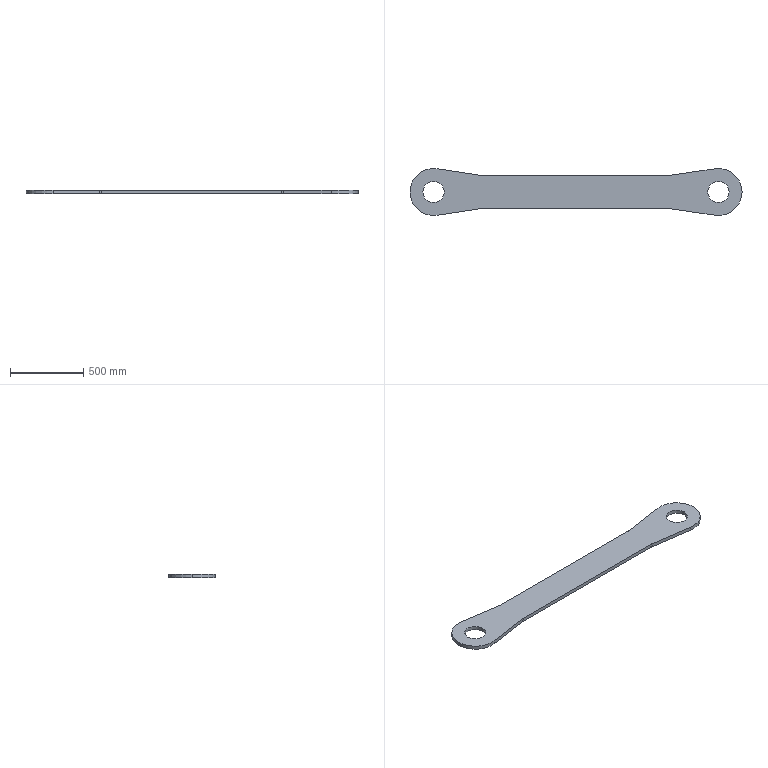Part | NX | features 前连杆 2 | 1 solid | 17 faces | box 2260 x 320 x 25 mm | volume 12756678 mm3 | cylinder 9 | plane 8 | commonest cylinder face diameters 200 x4 145 x2 320.239 x2 320 x1
STEP:
#1=CARTESIAN_POINT('',(-81.995,158.208,320.));
#2=VERTEX_POINT('',#1);
#3=CARTESIAN_POINT('',(-265.872,0.,320.));
#4=VERTEX_POINT('',#3);
#5=CARTESIAN_POINT('',(-105.752,-0.139,320.));
#6=DIRECTION('',(0.,0.,1.));
#7=DIRECTION('',(1.,0.,0.));
#8=AXIS2_PLACEMENT_3D('',#5,#6,#7);
#9=CIRCLE('',#8,160.12);
#10=EDGE_CURVE('',#2,#4,#9,.T.);
#11=ORIENTED_EDGE('',*,*,#10,.T.);
#12=CARTESIAN_POINT('',(-265.872,0.,345.));
#13=VERTEX_POINT('',#12);
#14=CARTESIAN_POINT('',(-265.872,0.,345.));
#15=DIRECTION('',(0.,0.,-1.));
#16=VECTOR('',#15,1000.);
#17=LINE('',#14,#16);
#18=EDGE_CURVE('',#13,#4,#17,.T.);
#19=ORIENTED_EDGE('',*,*,#18,.F.);
#20=CARTESIAN_POINT('',(-81.995,158.208,345.));
#21=VERTEX_POINT('',#20);
#22=CARTESIAN_POINT('',(-105.752,-0.139,345.));
#23=DIRECTION('',(0.,0.,1.));
#24=DIRECTION('',(1.,0.,0.));
#25=AXIS2_PLACEMENT_3D('',#22,#23,#24);
#26=CIRCLE('',#25,160.12);
#27=EDGE_CURVE('',#21,#13,#26,.T.);
#28=ORIENTED_EDGE('',*,*,#27,.F.);
#29=CARTESIAN_POINT('',(-81.995,158.208,345.));
#30=DIRECTION('',(0.,0.,-1.));
#31=VECTOR('',#30,1000.);
#32=LINE('',#29,#31);
#33=EDGE_CURVE('',#21,#2,#32,.T.);
#34=ORIENTED_EDGE('',*,*,#33,.T.);
#35=EDGE_LOOP('',(#11,#19,#28,#34));
#36=FACE_BOUND('',#35,.T.);
#37=CARTESIAN_POINT('',(-105.752,-0.139,345.));
#38=DIRECTION('',(0.,0.,-1.));
#39=DIRECTION('',(-1.,0.,0.));
#40=AXIS2_PLACEMENT_3D('',#37,#38,#39);
#41=CYLINDRICAL_SURFACE('',#40,160.12);
#42=ADVANCED_FACE('',(#36),#41,.T.);
#43=CARTESIAN_POINT('',(-81.995,-158.208,320.));
#44=VERTEX_POINT('',#43);
#45=CARTESIAN_POINT('',(-105.752,0.139,320.));
#46=DIRECTION('',(0.,0.,1.));
#47=DIRECTION('',(-1.,0.,0.));
#48=AXIS2_PLACEMENT_3D('',#45,#46,#47);
#49=CIRCLE('',#48,160.12);
#50=EDGE_CURVE('',#4,#44,#49,.T.);
#51=ORIENTED_EDGE('',*,*,#50,.T.);
#52=CARTESIAN_POINT('',(-81.995,-158.208,345.));
#53=VERTEX_POINT('',#52);
#54=CARTESIAN_POINT('',(-81.995,-158.208,345.));
#55=DIRECTION('',(0.,0.,-1.));
#56=VECTOR('',#55,1000.);
#57=LINE('',#54,#56);
#58=EDGE_CURVE('',#53,#44,#57,.T.);
#59=ORIENTED_EDGE('',*,*,#58,.F.);
#60=CARTESIAN_POINT('',(-105.752,0.139,345.));
#61=DIRECTION('',(0.,0.,1.));
#62=DIRECTION('',(-1.,0.,0.));
#63=AXIS2_PLACEMENT_3D('',#60,#61,#62);
#64=CIRCLE('',#63,160.12);
#65=EDGE_CURVE('',#13,#53,#64,.T.);
#66=ORIENTED_EDGE('',*,*,#65,.F.);
#67=ORIENTED_EDGE('',*,*,#18,.T.);
#68=EDGE_LOOP('',(#51,#59,#66,#67));
#69=FACE_BOUND('',#68,.T.);
#70=CARTESIAN_POINT('',(-105.752,0.139,345.));
#71=DIRECTION('',(0.,0.,-1.));
#72=DIRECTION('',(-1.,0.,0.));
#73=AXIS2_PLACEMENT_3D('',#70,#71,#72);
#74=CYLINDRICAL_SURFACE('',#73,160.12);
#75=ADVANCED_FACE('',(#69),#74,.T.);
#76=CARTESIAN_POINT('',(237.459,-110.28,320.));
#77=VERTEX_POINT('',#76);
#78=CARTESIAN_POINT('',(-81.995,-158.208,320.));
#79=DIRECTION('',(0.9889,0.1484,0.));
#80=VECTOR('',#79,1000.);
#81=LINE('',#78,#80);
#82=EDGE_CURVE('',#44,#77,#81,.T.);
#83=ORIENTED_EDGE('',*,*,#82,.T.);
#84=CARTESIAN_POINT('',(237.459,-110.28,345.));
#85=VERTEX_POINT('',#84);
#86=CARTESIAN_POINT('',(237.459,-110.28,345.));
#87=DIRECTION('',(0.,0.,-1.));
#88=VECTOR('',#87,1000.);
#89=LINE('',#86,#88);
#90=EDGE_CURVE('',#85,#77,#89,.T.);
#91=ORIENTED_EDGE('',*,*,#90,.F.);
#92=CARTESIAN_POINT('',(-81.995,-158.208,345.));
#93=DIRECTION('',(0.9889,0.1484,0.));
#94=VECTOR('',#93,1000.);
#95=LINE('',#92,#94);
#96=EDGE_CURVE('',#53,#85,#95,.T.);
#97=ORIENTED_EDGE('',*,*,#96,.F.);
#98=ORIENTED_EDGE('',*,*,#58,.T.);
#99=EDGE_LOOP('',(#83,#91,#97,#98));
#100=FACE_BOUND('',#99,.T.);
#101=CARTESIAN_POINT('',(-81.995,-158.208,345.));
#102=DIRECTION('',(-0.1484,0.9889,0.));
#103=DIRECTION('',(-0.9889,-0.1484,0.));
#104=AXIS2_PLACEMENT_3D('',#101,#102,#103);
#105=PLANE('',#104);
#106=ADVANCED_FACE('',(#100),#105,.F.);
#107=CARTESIAN_POINT('',(244.942,-110.,320.));
#108=VERTEX_POINT('',#107);
#109=CARTESIAN_POINT('',(244.942,-210.,320.));
#110=DIRECTION('',(0.,0.,-1.));
#111=DIRECTION('',(-1.,0.,0.));
#112=AXIS2_PLACEMENT_3D('',#109,#110,#111);
#113=CIRCLE('',#112,100.);
#114=EDGE_CURVE('',#77,#108,#113,.T.);
#115=ORIENTED_EDGE('',*,*,#114,.T.);
#116=CARTESIAN_POINT('',(244.942,-110.,345.));
#117=VERTEX_POINT('',#116);
#118=CARTESIAN_POINT('',(244.942,-110.,345.));
#119=DIRECTION('',(0.,0.,-1.));
#120=VECTOR('',#119,1000.);
#121=LINE('',#118,#120);
#122=EDGE_CURVE('',#117,#108,#121,.T.);
#123=ORIENTED_EDGE('',*,*,#122,.F.);
#124=CARTESIAN_POINT('',(244.942,-210.,345.));
#125=DIRECTION('',(0.,0.,-1.));
#126=DIRECTION('',(-1.,0.,0.));
#127=AXIS2_PLACEMENT_3D('',#124,#125,#126);
#128=CIRCLE('',#127,100.);
#129=EDGE_CURVE('',#85,#117,#128,.T.);
#130=ORIENTED_EDGE('',*,*,#129,.F.);
#131=ORIENTED_EDGE('',*,*,#90,.T.);
#132=EDGE_LOOP('',(#115,#123,#130,#131));
#133=FACE_BOUND('',#132,.T.);
#134=CARTESIAN_POINT('',(244.942,-210.,345.));
#135=DIRECTION('',(0.,0.,-1.));
#136=DIRECTION('',(-1.,0.,0.));
#137=AXIS2_PLACEMENT_3D('',#134,#135,#136);
#138=CYLINDRICAL_SURFACE('',#137,100.);
#139=ADVANCED_FACE('',(#133),#138,.F.);
#140=CARTESIAN_POINT('',(1473.599,-110.,320.));
#141=VERTEX_POINT('',#140);
#142=CARTESIAN_POINT('',(244.942,-110.,320.));
#143=DIRECTION('',(1.,0.,0.));
#144=VECTOR('',#143,1000.);
#145=LINE('',#142,#144);
#146=EDGE_CURVE('',#108,#141,#145,.T.);
#147=ORIENTED_EDGE('',*,*,#146,.T.);
#148=CARTESIAN_POINT('',(1473.599,-110.,345.));
#149=VERTEX_POINT('',#148);
#150=CARTESIAN_POINT('',(1473.599,-110.,345.));
#151=DIRECTION('',(0.,0.,-1.));
#152=VECTOR('',#151,1000.);
#153=LINE('',#150,#152);
#154=EDGE_CURVE('',#149,#141,#153,.T.);
#155=ORIENTED_EDGE('',*,*,#154,.F.);
#156=CARTESIAN_POINT('',(244.942,-110.,345.));
#157=DIRECTION('',(1.,0.,0.));
#158=VECTOR('',#157,1000.);
#159=LINE('',#156,#158);
#160=EDGE_CURVE('',#117,#149,#159,.T.);
#161=ORIENTED_EDGE('',*,*,#160,.F.);
#162=ORIENTED_EDGE('',*,*,#122,.T.);
#163=EDGE_LOOP('',(#147,#155,#161,#162));
#164=FACE_BOUND('',#163,.T.);
#165=CARTESIAN_POINT('',(244.942,-110.,345.));
#166=DIRECTION('',(0.,1.,0.));
#167=DIRECTION('',(0.,0.,1.));
#168=AXIS2_PLACEMENT_3D('',#165,#166,#167);
#169=PLANE('',#168);
#170=ADVANCED_FACE('',(#164),#169,.F.);
#171=CARTESIAN_POINT('',(1488.081,-111.054,320.));
#172=VERTEX_POINT('',#171);
#173=CARTESIAN_POINT('',(1473.599,-210.,320.));
#174=DIRECTION('',(0.,0.,-1.));
#175=DIRECTION('',(-1.,0.,0.));
#176=AXIS2_PLACEMENT_3D('',#173,#174,#175);
#177=CIRCLE('',#176,100.);
#178=EDGE_CURVE('',#141,#172,#177,.T.);
#179=ORIENTED_EDGE('',*,*,#178,.T.);
#180=CARTESIAN_POINT('',(1488.081,-111.054,345.));
#181=VERTEX_POINT('',#180);
#182=CARTESIAN_POINT('',(1488.081,-111.054,345.));
#183=DIRECTION('',(0.,0.,-1.));
#184=VECTOR('',#183,1000.);
#185=LINE('',#182,#184);
#186=EDGE_CURVE('',#181,#172,#185,.T.);
#187=ORIENTED_EDGE('',*,*,#186,.F.);
#188=CARTESIAN_POINT('',(1473.599,-210.,345.));
#189=DIRECTION('',(0.,0.,-1.));
#190=DIRECTION('',(-1.,0.,0.));
#191=AXIS2_PLACEMENT_3D('',#188,#189,#190);
#192=CIRCLE('',#191,100.);
#193=EDGE_CURVE('',#149,#181,#192,.T.);
#194=ORIENTED_EDGE('',*,*,#193,.F.);
#195=ORIENTED_EDGE('',*,*,#154,.T.);
#196=EDGE_LOOP('',(#179,#187,#194,#195));
#197=FACE_BOUND('',#196,.T.);
#198=CARTESIAN_POINT('',(1473.599,-210.,345.));
#199=DIRECTION('',(0.,0.,-1.));
#200=DIRECTION('',(-1.,0.,0.));
#201=AXIS2_PLACEMENT_3D('',#198,#199,#200);
#202=CYLINDRICAL_SURFACE('',#201,100.);
#203=ADVANCED_FACE('',(#197),#202,.F.);
#204=CARTESIAN_POINT('',(1810.956,-158.313,320.));
#205=VERTEX_POINT('',#204);
#206=CARTESIAN_POINT('',(1488.081,-111.054,320.));
#207=DIRECTION('',(0.9895,-0.1448,0.));
#208=VECTOR('',#207,1000.);
#209=LINE('',#206,#208);
#210=EDGE_CURVE('',#172,#205,#209,.T.);
#211=ORIENTED_EDGE('',*,*,#210,.T.);
#212=CARTESIAN_POINT('',(1810.956,-158.313,345.));
#213=VERTEX_POINT('',#212);
#214=CARTESIAN_POINT('',(1810.956,-158.313,345.));
#215=DIRECTION('',(0.,0.,-1.));
#216=VECTOR('',#215,1000.);
#217=LINE('',#214,#216);
#218=EDGE_CURVE('',#213,#205,#217,.T.);
#219=ORIENTED_EDGE('',*,*,#218,.F.);
#220=CARTESIAN_POINT('',(1488.081,-111.054,345.));
#221=DIRECTION('',(0.9895,-0.1448,0.));
#222=VECTOR('',#221,1000.);
#223=LINE('',#220,#222);
#224=EDGE_CURVE('',#181,#213,#223,.T.);
#225=ORIENTED_EDGE('',*,*,#224,.F.);
#226=ORIENTED_EDGE('',*,*,#186,.T.);
#227=EDGE_LOOP('',(#211,#219,#225,#226));
#228=FACE_BOUND('',#227,.T.);
#229=CARTESIAN_POINT('',(1488.081,-111.054,345.));
#230=DIRECTION('',(0.1448,0.9895,0.));
#231=DIRECTION('',(-0.9895,0.1448,0.));
#232=AXIS2_PLACEMENT_3D('',#229,#230,#231);
#233=PLANE('',#232);
#234=ADVANCED_FACE('',(#228),#233,.F.);
#235=CARTESIAN_POINT('',(1810.956,158.313,320.));
#236=VERTEX_POINT('',#235);
#237=CARTESIAN_POINT('',(1834.128,0.,320.));
#238=DIRECTION('',(0.,0.,1.));
#239=DIRECTION('',(-1.,0.,0.));
#240=AXIS2_PLACEMENT_3D('',#237,#238,#239);
#241=CIRCLE('',#240,160.);
#242=EDGE_CURVE('',#205,#236,#241,.T.);
#243=ORIENTED_EDGE('',*,*,#242,.T.);
#244=CARTESIAN_POINT('',(1810.956,158.313,345.));
#245=VERTEX_POINT('',#244);
#246=CARTESIAN_POINT('',(1810.956,158.313,345.));
#247=DIRECTION('',(0.,0.,-1.));
#248=VECTOR('',#247,1000.);
#249=LINE('',#246,#248);
#250=EDGE_CURVE('',#245,#236,#249,.T.);
#251=ORIENTED_EDGE('',*,*,#250,.F.);
#252=CARTESIAN_POINT('',(1834.128,0.,345.));
#253=DIRECTION('',(0.,0.,1.));
#254=DIRECTION('',(-1.,0.,0.));
#255=AXIS2_PLACEMENT_3D('',#252,#253,#254);
#256=CIRCLE('',#255,160.);
#257=EDGE_CURVE('',#213,#245,#256,.T.);
#258=ORIENTED_EDGE('',*,*,#257,.F.);
#259=ORIENTED_EDGE('',*,*,#218,.T.);
#260=EDGE_LOOP('',(#243,#251,#258,#259));
#261=FACE_BOUND('',#260,.T.);
#262=CARTESIAN_POINT('',(1834.128,0.,345.));
#263=DIRECTION('',(0.,0.,-1.));
#264=DIRECTION('',(-1.,0.,0.));
#265=AXIS2_PLACEMENT_3D('',#262,#263,#264);
#266=CYLINDRICAL_SURFACE('',#265,160.);
#267=ADVANCED_FACE('',(#261),#266,.T.);
#268=CARTESIAN_POINT('',(1488.081,111.054,320.));
#269=VERTEX_POINT('',#268);
#270=CARTESIAN_POINT('',(1488.081,111.054,320.));
#271=DIRECTION('',(-0.9895,-0.1448,0.));
#272=VECTOR('',#271,1000.);
#273=LINE('',#270,#272);
#274=EDGE_CURVE('',#236,#269,#273,.T.);
#275=ORIENTED_EDGE('',*,*,#274,.T.);
#276=CARTESIAN_POINT('',(1488.081,111.054,345.));
#277=VERTEX_POINT('',#276);
#278=CARTESIAN_POINT('',(1488.081,111.054,345.));
#279=DIRECTION('',(0.,0.,-1.));
#280=VECTOR('',#279,1000.);
#281=LINE('',#278,#280);
#282=EDGE_CURVE('',#277,#269,#281,.T.);
#283=ORIENTED_EDGE('',*,*,#282,.F.);
#284=CARTESIAN_POINT('',(1488.081,111.054,345.));
#285=DIRECTION('',(-0.9895,-0.1448,0.));
#286=VECTOR('',#285,1000.);
#287=LINE('',#284,#286);
#288=EDGE_CURVE('',#245,#277,#287,.T.);
#289=ORIENTED_EDGE('',*,*,#288,.F.);
#290=ORIENTED_EDGE('',*,*,#250,.T.);
#291=EDGE_LOOP('',(#275,#283,#289,#290));
#292=FACE_BOUND('',#291,.T.);
#293=CARTESIAN_POINT('',(1488.081,111.054,345.));
#294=DIRECTION('',(0.1448,-0.9895,0.));
#295=DIRECTION('',(0.9895,0.1448,0.));
#296=AXIS2_PLACEMENT_3D('',#293,#294,#295);
#297=PLANE('',#296);
#298=ADVANCED_FACE('',(#292),#297,.F.);
#299=CARTESIAN_POINT('',(1473.599,110.,320.));
#300=VERTEX_POINT('',#299);
#301=CARTESIAN_POINT('',(1473.599,210.,320.));
#302=DIRECTION('',(0.,0.,-1.));
#303=DIRECTION('',(1.,0.,0.));
#304=AXIS2_PLACEMENT_3D('',#301,#302,#303);
#305=CIRCLE('',#304,100.);
#306=EDGE_CURVE('',#269,#300,#305,.T.);
#307=ORIENTED_EDGE('',*,*,#306,.T.);
#308=CARTESIAN_POINT('',(1473.599,110.,345.));
#309=VERTEX_POINT('',#308);
#310=CARTESIAN_POINT('',(1473.599,110.,345.));
#311=DIRECTION('',(0.,0.,-1.));
#312=VECTOR('',#311,1000.);
#313=LINE('',#310,#312);
#314=EDGE_CURVE('',#309,#300,#313,.T.);
#315=ORIENTED_EDGE('',*,*,#314,.F.);
#316=CARTESIAN_POINT('',(1473.599,210.,345.));
#317=DIRECTION('',(0.,0.,-1.));
#318=DIRECTION('',(1.,0.,0.));
#319=AXIS2_PLACEMENT_3D('',#316,#317,#318);
#320=CIRCLE('',#319,100.);
#321=EDGE_CURVE('',#277,#309,#320,.T.);
#322=ORIENTED_EDGE('',*,*,#321,.F.);
#323=ORIENTED_EDGE('',*,*,#282,.T.);
#324=EDGE_LOOP('',(#307,#315,#322,#323));
#325=FACE_BOUND('',#324,.T.);
#326=CARTESIAN_POINT('',(1473.599,210.,345.));
#327=DIRECTION('',(0.,0.,-1.));
#328=DIRECTION('',(-1.,0.,0.));
#329=AXIS2_PLACEMENT_3D('',#326,#327,#328);
#330=CYLINDRICAL_SURFACE('',#329,100.);
#331=ADVANCED_FACE('',(#325),#330,.F.);
#332=CARTESIAN_POINT('',(244.942,110.,320.));
#333=VERTEX_POINT('',#332);
#334=CARTESIAN_POINT('',(244.942,110.,320.));
#335=DIRECTION('',(-1.,0.,0.));
#336=VECTOR('',#335,1000.);
#337=LINE('',#334,#336);
#338=EDGE_CURVE('',#300,#333,#337,.T.);
#339=ORIENTED_EDGE('',*,*,#338,.T.);
#340=CARTESIAN_POINT('',(244.942,110.,345.));
#341=VERTEX_POINT('',#340);
#342=CARTESIAN_POINT('',(244.942,110.,345.));
#343=DIRECTION('',(0.,0.,-1.));
#344=VECTOR('',#343,1000.);
#345=LINE('',#342,#344);
#346=EDGE_CURVE('',#341,#333,#345,.T.);
#347=ORIENTED_EDGE('',*,*,#346,.F.);
#348=CARTESIAN_POINT('',(244.942,110.,345.));
#349=DIRECTION('',(-1.,0.,0.));
#350=VECTOR('',#349,1000.);
#351=LINE('',#348,#350);
#352=EDGE_CURVE('',#309,#341,#351,.T.);
#353=ORIENTED_EDGE('',*,*,#352,.F.);
#354=ORIENTED_EDGE('',*,*,#314,.T.);
#355=EDGE_LOOP('',(#339,#347,#353,#354));
#356=FACE_BOUND('',#355,.T.);
#357=CARTESIAN_POINT('',(244.942,110.,345.));
#358=DIRECTION('',(0.,-1.,0.));
#359=DIRECTION('',(1.,0.,0.));
#360=AXIS2_PLACEMENT_3D('',#357,#358,#359);
#361=PLANE('',#360);
#362=ADVANCED_FACE('',(#356),#361,.F.);
#363=CARTESIAN_POINT('',(237.459,110.28,320.));
#364=VERTEX_POINT('',#363);
#365=CARTESIAN_POINT('',(244.942,210.,320.));
#366=DIRECTION('',(0.,0.,-1.));
#367=DIRECTION('',(1.,0.,0.));
#368=AXIS2_PLACEMENT_3D('',#365,#366,#367);
#369=CIRCLE('',#368,100.);
#370=EDGE_CURVE('',#333,#364,#369,.T.);
#371=ORIENTED_EDGE('',*,*,#370,.T.);
#372=CARTESIAN_POINT('',(237.459,110.28,345.));
#373=VERTEX_POINT('',#372);
#374=CARTESIAN_POINT('',(237.459,110.28,345.));
#375=DIRECTION('',(0.,0.,-1.));
#376=VECTOR('',#375,1000.);
#377=LINE('',#374,#376);
#378=EDGE_CURVE('',#373,#364,#377,.T.);
#379=ORIENTED_EDGE('',*,*,#378,.F.);
#380=CARTESIAN_POINT('',(244.942,210.,345.));
#381=DIRECTION('',(0.,0.,-1.));
#382=DIRECTION('',(1.,0.,0.));
#383=AXIS2_PLACEMENT_3D('',#380,#381,#382);
#384=CIRCLE('',#383,100.);
#385=EDGE_CURVE('',#341,#373,#384,.T.);
#386=ORIENTED_EDGE('',*,*,#385,.F.);
#387=ORIENTED_EDGE('',*,*,#346,.T.);
#388=EDGE_LOOP('',(#371,#379,#386,#387));
#389=FACE_BOUND('',#388,.T.);
#390=CARTESIAN_POINT('',(244.942,210.,345.));
#391=DIRECTION('',(0.,0.,-1.));
#392=DIRECTION('',(-1.,0.,0.));
#393=AXIS2_PLACEMENT_3D('',#390,#391,#392);
#394=CYLINDRICAL_SURFACE('',#393,100.);
#395=ADVANCED_FACE('',(#389),#394,.F.);
#396=CARTESIAN_POINT('',(-81.995,158.208,320.));
#397=DIRECTION('',(-0.9889,0.1484,0.));
#398=VECTOR('',#397,1000.);
#399=LINE('',#396,#398);
#400=EDGE_CURVE('',#364,#2,#399,.T.);
#401=ORIENTED_EDGE('',*,*,#400,.T.);
#402=ORIENTED_EDGE('',*,*,#33,.F.);
#403=CARTESIAN_POINT('',(-81.995,158.208,345.));
#404=DIRECTION('',(-0.9889,0.1484,0.));
#405=VECTOR('',#404,1000.);
#406=LINE('',#403,#405);
#407=EDGE_CURVE('',#373,#21,#406,.T.);
#408=ORIENTED_EDGE('',*,*,#407,.F.);
#409=ORIENTED_EDGE('',*,*,#378,.T.);
#410=EDGE_LOOP('',(#401,#402,#408,#409));
#411=FACE_BOUND('',#410,.T.);
#412=CARTESIAN_POINT('',(-81.995,158.208,345.));
#413=DIRECTION('',(-0.1484,-0.9889,0.));
#414=DIRECTION('',(0.9889,-0.1484,0.));
#415=AXIS2_PLACEMENT_3D('',#412,#413,#414);
#416=PLANE('',#415);
#417=ADVANCED_FACE('',(#411),#416,.F.);
#418=CARTESIAN_POINT('',(-178.372,0.,345.));
#419=VERTEX_POINT('',#418);
#420=CARTESIAN_POINT('',(-105.872,0.,345.));
#421=DIRECTION('',(0.,0.,-1.));
#422=DIRECTION('',(-1.,0.,0.));
#423=AXIS2_PLACEMENT_3D('',#420,#421,#422);
#424=CIRCLE('',#423,72.5);
#425=EDGE_CURVE('',#419,#419,#424,.T.);
#426=ORIENTED_EDGE('',*,*,#425,.T.);
#427=EDGE_LOOP('',(#426));
#428=FACE_BOUND('',#427,.T.);
#429=CARTESIAN_POINT('',(1761.628,0.,345.));
#430=VERTEX_POINT('',#429);
#431=CARTESIAN_POINT('',(1834.128,0.,345.));
#432=DIRECTION('',(0.,0.,-1.));
#433=DIRECTION('',(-1.,0.,0.));
#434=AXIS2_PLACEMENT_3D('',#431,#432,#433);
#435=CIRCLE('',#434,72.5);
#436=EDGE_CURVE('',#430,#430,#435,.T.);
#437=ORIENTED_EDGE('',*,*,#436,.T.);
#438=EDGE_LOOP('',(#437));
#439=FACE_BOUND('',#438,.T.);
#440=ORIENTED_EDGE('',*,*,#27,.T.);
#441=ORIENTED_EDGE('',*,*,#65,.T.);
#442=ORIENTED_EDGE('',*,*,#96,.T.);
#443=ORIENTED_EDGE('',*,*,#129,.T.);
#444=ORIENTED_EDGE('',*,*,#160,.T.);
#445=ORIENTED_EDGE('',*,*,#193,.T.);
#446=ORIENTED_EDGE('',*,*,#224,.T.);
#447=ORIENTED_EDGE('',*,*,#257,.T.);
#448=ORIENTED_EDGE('',*,*,#288,.T.);
#449=ORIENTED_EDGE('',*,*,#321,.T.);
#450=ORIENTED_EDGE('',*,*,#352,.T.);
#451=ORIENTED_EDGE('',*,*,#385,.T.);
#452=ORIENTED_EDGE('',*,*,#407,.T.);
#453=EDGE_LOOP('',(#440,#441,#442,#443,#444,#445,#446,#447,#448,#449,#450,#451,#452));
#454=FACE_BOUND('',#453,.T.);
#455=CARTESIAN_POINT('',(-105.752,-0.139,345.));
#456=DIRECTION('',(0.,0.,1.));
#457=DIRECTION('',(1.,0.,0.));
#458=AXIS2_PLACEMENT_3D('',#455,#456,#457);
#459=PLANE('',#458);
#460=ADVANCED_FACE('',(#428,#439,#454),#459,.T.);
#461=CARTESIAN_POINT('',(-33.372,0.,320.));
#462=VERTEX_POINT('',#461);
#463=CARTESIAN_POINT('',(-105.872,0.,320.));
#464=DIRECTION('',(0.,0.,1.));
#465=DIRECTION('',(1.,0.,0.));
#466=AXIS2_PLACEMENT_3D('',#463,#464,#465);
#467=CIRCLE('',#466,72.5);
#468=EDGE_CURVE('',#462,#462,#467,.T.);
#469=ORIENTED_EDGE('',*,*,#468,.T.);
#470=EDGE_LOOP('',(#469));
#471=FACE_BOUND('',#470,.T.);
#472=CARTESIAN_POINT('',(1906.628,0.,320.));
#473=VERTEX_POINT('',#472);
#474=CARTESIAN_POINT('',(1834.128,0.,320.));
#475=DIRECTION('',(0.,0.,1.));
#476=DIRECTION('',(1.,0.,0.));
#477=AXIS2_PLACEMENT_3D('',#474,#475,#476);
#478=CIRCLE('',#477,72.5);
#479=EDGE_CURVE('',#473,#473,#478,.T.);
#480=ORIENTED_EDGE('',*,*,#479,.T.);
#481=EDGE_LOOP('',(#480));
#482=FACE_BOUND('',#481,.T.);
#483=ORIENTED_EDGE('',*,*,#10,.F.);
#484=ORIENTED_EDGE('',*,*,#400,.F.);
#485=ORIENTED_EDGE('',*,*,#370,.F.);
#486=ORIENTED_EDGE('',*,*,#338,.F.);
#487=ORIENTED_EDGE('',*,*,#306,.F.);
#488=ORIENTED_EDGE('',*,*,#274,.F.);
#489=ORIENTED_EDGE('',*,*,#242,.F.);
#490=ORIENTED_EDGE('',*,*,#210,.F.);
#491=ORIENTED_EDGE('',*,*,#178,.F.);
#492=ORIENTED_EDGE('',*,*,#146,.F.);
#493=ORIENTED_EDGE('',*,*,#114,.F.);
#494=ORIENTED_EDGE('',*,*,#82,.F.);
#495=ORIENTED_EDGE('',*,*,#50,.F.);
#496=EDGE_LOOP('',(#483,#484,#485,#486,#487,#488,#489,#490,#491,#492,#493,#494,#495));
#497=FACE_BOUND('',#496,.T.);
#498=CARTESIAN_POINT('',(-105.752,-0.139,320.));
#499=DIRECTION('',(0.,0.,1.));
#500=DIRECTION('',(1.,0.,0.));
#501=AXIS2_PLACEMENT_3D('',#498,#499,#500);
#502=PLANE('',#501);
#503=ADVANCED_FACE('',(#471,#482,#497),#502,.F.);
#504=ORIENTED_EDGE('',*,*,#436,.F.);
#505=EDGE_LOOP('',(#504));
#506=FACE_BOUND('',#505,.T.);
#507=ORIENTED_EDGE('',*,*,#479,.F.);
#508=EDGE_LOOP('',(#507));
#509=FACE_BOUND('',#508,.T.);
#510=CARTESIAN_POINT('',(1834.128,0.,345.));
#511=DIRECTION('',(0.,0.,-1.));
#512=DIRECTION('',(-1.,0.,0.));
#513=AXIS2_PLACEMENT_3D('',#510,#511,#512);
#514=CYLINDRICAL_SURFACE('',#513,72.5);
#515=ADVANCED_FACE('',(#506,#509),#514,.F.);
#516=ORIENTED_EDGE('',*,*,#425,.F.);
#517=EDGE_LOOP('',(#516));
#518=FACE_BOUND('',#517,.T.);
#519=ORIENTED_EDGE('',*,*,#468,.F.);
#520=EDGE_LOOP('',(#519));
#521=FACE_BOUND('',#520,.T.);
#522=CARTESIAN_POINT('',(-105.872,0.,345.));
#523=DIRECTION('',(0.,0.,-1.));
#524=DIRECTION('',(-1.,0.,0.));
#525=AXIS2_PLACEMENT_3D('',#522,#523,#524);
#526=CYLINDRICAL_SURFACE('',#525,72.5);
#527=ADVANCED_FACE('',(#518,#521),#526,.F.);
#528=CLOSED_SHELL('',(#42,#75,#106,#139,#170,#203,#234,#267,#298,#331,#362,#395,#417,#460,#503,#515,#527));
#529=MANIFOLD_SOLID_BREP('',#528);
#530=(LENGTH_UNIT()NAMED_UNIT(*)SI_UNIT(.MILLI.,.METRE.));
#531=UNCERTAINTY_MEASURE_WITH_UNIT(LENGTH_MEASURE(0.00001),#530,'','');
#532=(NAMED_UNIT(*)PLANE_ANGLE_UNIT()SI_UNIT($,.RADIAN.));
#533=(NAMED_UNIT(*)SI_UNIT($,.STERADIAN.)SOLID_ANGLE_UNIT());
#534=(GEOMETRIC_REPRESENTATION_CONTEXT(3)GLOBAL_UNCERTAINTY_ASSIGNED_CONTEXT((#531))GLOBAL_UNIT_ASSIGNED_CONTEXT((#530,#532,#533))REPRESENTATION_CONTEXT('',''));
#535=ADVANCED_BREP_SHAPE_REPRESENTATION('',(#529),#534);